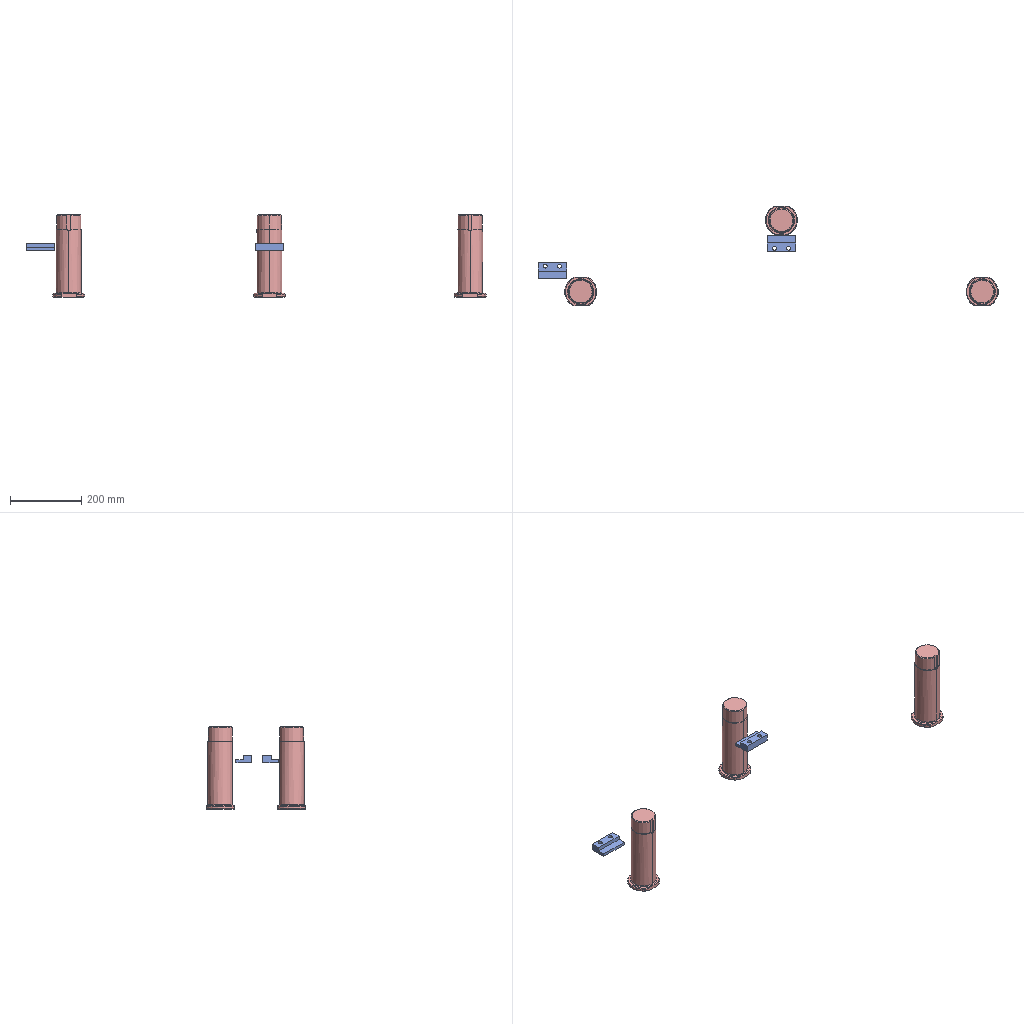Assembly | SolidWorks | 7 different items | 12 placed | box 1288 x 280 x 230 mm
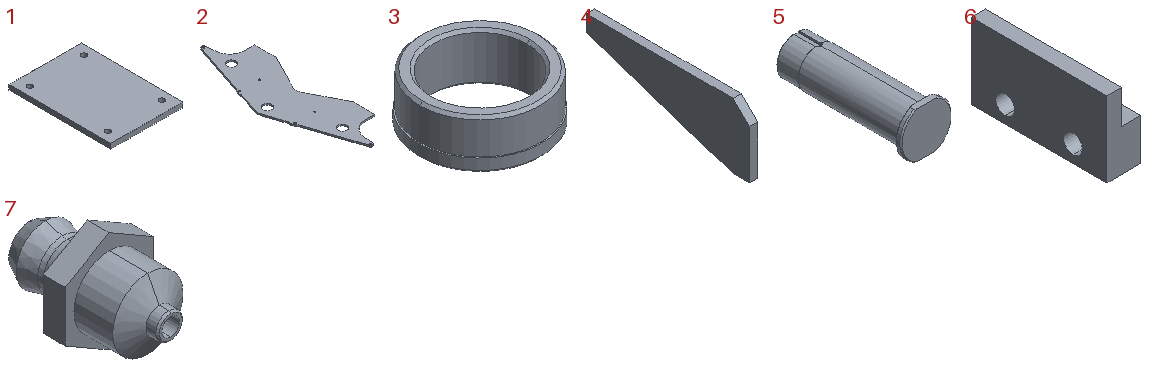Parts list (item | quantity | size | volume | features):
1 | x1 | 240 x 340 x 16 mm | 1289314 mm3 | features Extrusion 1
2 | x1 | 575.631 x 1726 x 16 mm | 8635461 mm3 | features Extrusion 1, HoleWzd 1, ICE 1
3 | x2 | 92 x 92 x 36 mm | 91314 mm3 | features Chamfer 1, Revolution 1
4 | x1 | 10 x 200 x 80 mm | 104000 mm3 | features Extrusion 1
5 | x3 | 90 x 230 x 80 mm | 896064 mm3 | features Fillet 3, ICE 2, Chamfer 1, Revolution 1
6 | x2 | 20 x 80 x 44.5 mm | 48999 mm3 | features Extrusion 1, ICE 1
7 | x2 | 10 x 16 x 11.547 mm | 627.343 mm3 | features Boss 1, Chamfer 1, Revolution 1
Mates (type | each side: item.copy, entity, surface, feature):
Coincident | 5.1 face plane Revolve1 | 5.2 face plane Revolve1
Coincident | 5.1 face plane Revolve1 | 5.3 face plane Revolve1
DistanceDim | 2.1 face plane Boss-Extrude1 | 1.1 face plane Boss-Extrude1
Coincident | 1.1 face plane Boss-Extrude1 | 2.1 face plane Boss-Extrude1
Coincident | 1.1 face plane Boss-Extrude1 | 4.1 face plane Boss-Extrude1
Coincident | 2.1 face plane Boss-Extrude1 | 4.1 face plane Boss-Extrude1
DistanceDim | 4.1 face plane Boss-Extrude1 | 2.1 face plane Boss-Extrude1
Concentric | 2.1 face cylinder Boss-Extrude1 | 3.1 face cylinder Revolve1
Coincident | 2.1 face plane Boss-Extrude1 | 3.1 face plane Revolve1
Concentric | 2.1 face cylinder Boss-Extrude1 | 3.2 face cylinder Revolve1
Coincident | 2.1 face plane Boss-Extrude1 | 3.2 face plane Revolve1
Coincident | 1.1 face plane Boss-Extrude1 | assembly plane
Parallel | 1.1 face plane Boss-Extrude1 | 5.3 face plane Cut-Extrude1
Concentric | 3.1 face cylinder Revolve1 | 5.3 face cylinder Revolve1
Parallel | 5.1 face plane Cut-Extrude1 | 6.1 face plane Boss-Extrude1
Parallel | 5.3 face plane Cut-Extrude1 | 6.2 face plane Boss-Extrude2